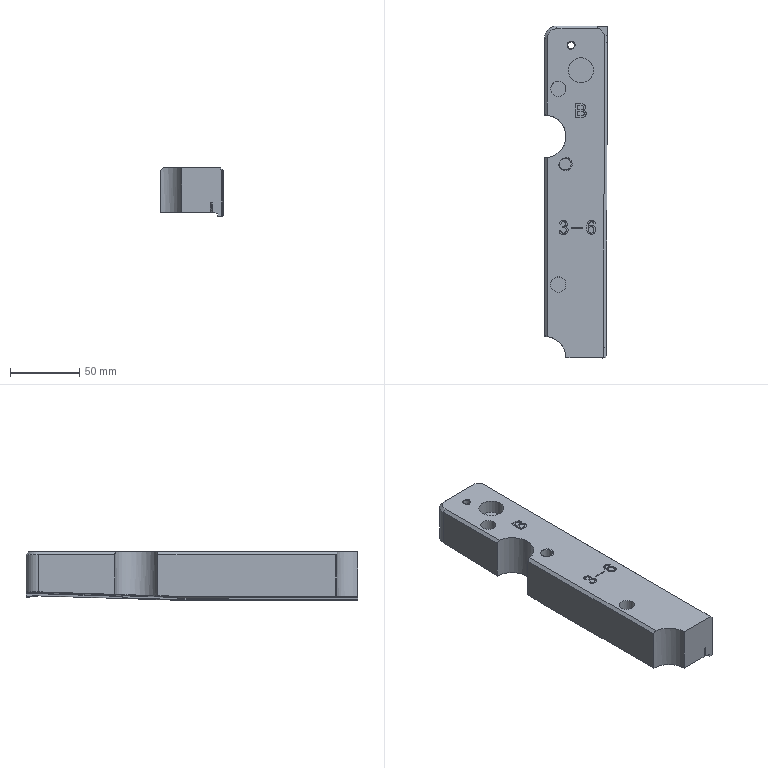NC program | NX | posted with a generic post | part box 45.476 x 239.737 x 35.001 mm
Lines 137 to 1068 of 14047:
(ZLEVEL_PROFILE , TOOL : D8R0.5)
N272 M6
N274 G53
N276 G17 G0 G90 X-123.905 Y28.641 S4500 M3
N278 G43 Z60. H0
N280 G94 G1 Z35.002 F4000.
N282 Z34.802 F1380.
N284 G3 X-120.891 Y25.655 R3.
N286 G1 X-119.898 Y25.659 F2300.
N288 X-119.885 Y25.662
N290 X-112.151 Y25.703
N292 X32.762 Y26.385
N294 X39.171 Y26.415 Z34.603 F100.
N296 X-112.151 Y25.703 F2300.
N298 X-119.885 Y25.662
N300 X-119.898 Y25.659
N302 X-120.891 Y25.655
N304 Z34.405 F100.
N306 X-119.89 Y25.662 F2300.
N308 X-112.153 Y25.703
N310 X-112.15
N312 X45.587 Y26.445
N314 X52.001 Y26.475 Z34.206 F100.
N316 X-112.15 Y25.703 F2300.
N318 X-112.153
N320 X-119.89 Y25.662
N322 X-120.891 Y25.655
N324 Z34.007 F100.
N326 X-119.89 Y25.662 F2300.
N328 X-112.153 Y25.703
N330 X-112.15
N332 X58.422 Y26.506
N334 X64.831 Y26.536 Z33.809 F100.
N336 X-112.15 Y25.703 F2300.
N338 X-112.153
N340 X-119.89 Y25.662
N342 X-120.891 Y25.655
N344 Z33.61 F100.
N346 X-119.89 Y25.662 F2300.
N348 X-112.153 Y25.703
N350 X-112.15
N352 X71.252 Y26.566
N354 X77.673 Y26.596 Z33.411 F100.
N356 X-112.15 Y25.703 F2300.
N358 X-112.153
N360 X-119.89 Y25.662
N362 X-120.891 Y25.655
N364 Z33.212 F100.
N366 X-119.89 Y25.662 F2300.
N368 X-112.153 Y25.703
N370 X-112.15
N372 X84.082 Y26.626
N374 G3 X87.068 Y29.64 R3.
N376 G1 Z33.412
N378 G0 Z60.
N380 X113.932 Y29.432
N382 G1 Z33.611 F4000.
N384 Z33.411 F1380.
N386 G3 X117.138 Y26.653 R3.
N388 G2 X119.632 Y26.738 R33.898 F2300.
N390 G1 X119.876
N392 G2 X123.869 Y22.744 R4.005
N394 G1 Y20.236
N396 G2 X123.582 Y18.314 R5.483
N398 X121.243 Y15.885 R4.013
N400 X116.883 Y17.033 R3.835
N402 X115.98 Y18.934 R4.396
N404 X114.06 Y19.41 R6.752
N406 X114.436 Y26.228 R3.615
N408 X116.388 Y26.591 R10.395
N410 X117.138 Y26.653 R33.898
N412 G1 X117.137 Y26.701 Z33.312 F100.
N414 X117.136 Y26.73 Z33.212
N416 G3 X114.789 Y26.601 R34.9 F2300.
N418 X112.765 Y26.236 R11.122
N420 X110.314 Y23.897 R3.595
N422 X112.79 Y19.251 R3.642
N424 G1 X113.253 Y19.112
N426 G3 X115.393 Y18.828 R13.686
N428 G2 X115.969 Y18.713 R2.024
N430 G3 X116.704 Y17.053 R4.135
N432 G1 X116.725 Y17.023
N434 G3 X123.156 Y17.227 R3.915
N436 X123.869 Y19.697 R4.438
N438 G1 Y22.744
N440 G3 X119.876 Y26.738 R4.005
N442 G1 X117.927
N444 G3 X117.136 Y26.73 R34.9
N446 G2 X114.073 Y29.666 R3.
N448 G1 Z33.412
N450 G0 Z33.611
N452 X-123.912 Y28.633
N454 G1 Z33.214 F4000.
N456 Z33.014 F1380.
N458 G3 X-120.891 Y25.655 R3.
N460 G1 X-119.89 Y25.662 F2300.
N462 X-112.153 Y25.703
N464 X-112.15
N466 X90.503 Y26.657
N468 G2 X103.915 Y26.501 R353.898
N470 X106.876 Y26.29 R36.623
N472 G1 X108.206 Y25.891
N474 G3 X109.592 Y25.363 R1.248
N476 G2 X111.274 Y26.29 R3.979
N478 X112.79 Y26.566 R9.709
N480 X116.229 Y26.738 R30.698
N482 G1 X119.876
N484 G2 X123.869 Y22.744 R4.005
N486 G1 Y19.437
N488 Y19.266 Z32.815 F100.
N490 Y22.744 F2300.
N492 G3 X119.876 Y26.738 R4.005
N494 G1 X114.527
N496 G3 X110.791 Y26.526 R28.567
N498 G1 X110.391 Y26.513
N500 X108.392 Y26.592
N502 G3 X96.912 Y26.687 R397.63
N504 G1 X-112.15 Y25.703
N506 X-112.153
N508 X-119.89 Y25.662
N510 X-120.891 Y25.655
N512 Z32.616 F100.
N514 X-119.89 Y25.662 F2300.
N516 X-112.153 Y25.703
N518 X-112.15
N520 X103.333 Y26.717
N522 G2 X110.791 Y26.683 R422.317
N524 X112.84 Y26.738 R49.109
N526 G1 X119.876
N528 G2 X123.869 Y22.744 R4.005
N530 G1 Y19.147
N532 Y19.053 Z32.418 F100.
N534 Y22.738 F2300.
N536 G3 X119.869 Y26.738 R4.
N538 G1 X107.859
N540 X-112.15 Y25.703
N542 X-112.153
N544 X-119.89 Y25.662
N546 X-120.891 Y25.655
N548 Z32.219 F100.
N550 X-119.89 Y25.662 F2300.
N552 X-112.153 Y25.703
N554 X-112.15
N556 X107.859 Y26.738
N558 X119.869
N560 G2 X123.869 Y22.738 R4.
N562 G1 Y19.011
N564 Y18.982 Z32.052 F100.
N566 Y22.738 F2300.
N568 G3 X119.869 Y26.738 R4.
N570 G1 X107.859
N572 X-112.15 Y25.703
N574 X-112.153
N576 X-119.89 Y25.662
N578 X-120.891 Y25.655
N580 Z31.886 F100.
N582 X-119.89 Y25.662 F2300.
N584 X-112.153 Y25.703
N586 X-112.15
N588 X107.859 Y26.738
N590 X119.869
N592 G2 X123.869 Y22.738 R4.
N594 G1 Y18.969
N596 Z31.719 F100.
N598 Y22.738 F2300.
N600 G3 X119.869 Y26.738 R4.
N602 G1 X107.859
N604 X-112.15 Y25.703
N606 X-112.153
N608 X-119.89 Y25.662
N610 X-120.891 Y25.655
N612 Z31.527 F100.
N614 X-119.89 Y25.662 F2300.
N616 X-112.153 Y25.703
N618 X-112.15
N620 X107.859 Y26.738
N622 X119.869
N624 G2 X123.869 Y22.738 R4.
N626 G1 Y18.969
N628 Z31.335 F100.
N630 Y22.738 F2300.
N632 G3 X119.869 Y26.738 R4.
N634 G1 X107.869
N636 X107.85
N638 X-112.15 Y25.703
N640 X-112.153
N642 X-119.89 Y25.662
N644 X-120.891 Y25.655
N646 Z31.143 F100.
N648 X-119.89 Y25.662 F2300.
N650 X-112.153 Y25.703
N652 X-112.15
N654 X107.85 Y26.738
N656 X107.869
N658 X119.869
N660 G2 X123.869 Y22.738 R4.
N662 G1 Y18.969
N664 Z30.951 F100.
N666 Y22.738 F2300.
N668 G3 X119.869 Y26.738 R4.
N670 G1 X107.869
N672 X107.85
N674 X-112.15 Y25.703
N676 X-112.153
N678 X-119.89 Y25.662
N680 X-120.891 Y25.655
N682 Z30.759 F100.
N684 X-119.89 Y25.662 F2300.
N686 X-112.153 Y25.703
N688 X-112.15
N690 X107.85 Y26.738
N692 X107.869
N694 X119.869
N696 G2 X123.869 Y22.738 R4.
N698 G1 Y18.969
N700 Z30.568 F100.
N702 Y22.738 F2300.
N704 G3 X119.869 Y26.738 R4.
N706 G1 X107.869
N708 X107.85
N710 X-112.15 Y25.703
N712 X-112.153
N714 X-119.89 Y25.662
N716 X-120.891 Y25.655
N718 Z30.376 F100.
N720 X-119.89 Y25.662 F2300.
N722 X-112.153 Y25.703
N724 X-112.15
N726 X107.85 Y26.738
N728 X107.869
N730 X119.869
N732 G2 X123.869 Y22.738 R4.
N734 G1 Y18.969
N736 X123.868 Y18.847 Z30.28 F100.
N738 X123.869 Y18.726 Z30.184
N740 Y22.738 F2300.
N742 G3 X119.869 Y26.738 R4.
N744 G1 X107.869
N746 X107.85
N748 X-112.15 Y25.703
N750 X-112.153
N752 X-119.89 Y25.662
N754 X-120.891 Y25.655
N756 Z29.992 F100.
N758 X-119.89 Y25.662 F2300.
N760 X-112.153 Y25.703
N762 X-112.15
N764 X107.85 Y26.738
N766 X107.869
N768 X119.869
N770 G2 X123.869 Y22.738 R4.
N772 G1 Y17.667
N774 Y16.591 Z29.8 F100.
N776 Y22.738 F2300.
N778 G3 X119.869 Y26.738 R4.
N780 G1 X107.869
N782 X107.85
N784 X-112.15 Y25.703
N786 X-112.153
N788 X-119.89 Y25.662
N790 X-120.891 Y25.655
N792 Z29.608 F100.
N794 X-119.89 Y25.662 F2300.
N796 X-112.153 Y25.703
N798 X-112.15
N800 X107.85 Y26.738
N802 X107.869
N804 X119.869
N806 G2 X123.869 Y22.738 R4.
N808 G1 Y15.342
N810 G2 X119.86 Y11.53 R4.009
N812 G1 X110.056
N814 X109.498 Z29.416 F100.
N816 X119.86 F2300.
N818 G3 X123.869 Y15.342 R4.009
N820 G1 Y22.738
N822 G3 X119.869 Y26.738 R4.
N824 G1 X107.869
N826 X107.85
N828 X-112.15 Y25.703
N830 X-112.153
N832 X-119.89 Y25.662
N834 X-120.891 Y25.655
N836 G2 X-123.912 Y28.634 R3.
N838 G1 Z29.616
N840 G0 Z60.
N842 X-111.361 Y-26.73
N844 G1 Z32.816 F4000.
N846 Z32.616 F1380.
N848 G3 X-108.366 Y-23.725 R3.
N850 G1 X-108.368 Y-22.722 F2300.
N852 G3 X-119.868 Y-11.238 R11.502
N854 G1 X-120.866 Y-11.236
N856 Z32.418 F100.
N858 X-119.868 Y-11.238 F2300.
N860 G2 X-108.368 Y-22.722 R11.502
N862 G1 X-108.366 Y-23.725
N864 Z32.219 F100.
N866 X-108.368 Y-22.722 F2300.
N868 G3 X-119.868 Y-11.238 R11.502
N870 G1 X-120.866 Y-11.236
N872 Z32.052 F100.
N874 X-119.868 Y-11.238 F2300.
N876 G2 X-108.368 Y-22.722 R11.502
N878 G1 X-108.366 Y-23.725
N880 Z31.886 F100.
N882 X-108.368 Y-22.722 F2300.
N884 G3 X-119.868 Y-11.238 R11.502
N886 G1 X-120.866 Y-11.236
N888 Z31.719 F100.
N890 X-119.868 Y-11.238 F2300.
N892 G2 X-108.368 Y-22.722 R11.502
N894 G1 X-108.366 Y-23.725
N896 Z31.527 F100.
N898 X-108.368 Y-22.759 F2300.
N900 X-108.369 Y-22.73
N902 G3 X-119.869 Y-11.238 R11.5
N904 G1 X-120.866 Y-11.236
N906 Z31.335 F100.
N908 X-119.869 Y-11.238 F2300.
N910 G2 X-108.369 Y-22.73 R11.5
N912 G1 X-108.368 Y-22.759
N914 X-108.366 Y-23.725
N916 Z31.143 F100.
N918 X-108.368 Y-22.759 F2300.
N920 X-108.369 Y-22.73
N922 G3 X-119.869 Y-11.238 R11.5
N924 G1 X-120.866 Y-11.236
N926 Z30.951 F100.
N928 X-119.869 Y-11.238 F2300.
N930 G2 X-108.369 Y-22.73 R11.5
N932 G1 X-108.368 Y-22.759
N934 X-108.366 Y-23.725
N936 Z30.759 F100.
N938 X-108.368 Y-22.759 F2300.
N940 X-108.369 Y-22.73
N942 G3 X-119.869 Y-11.238 R11.5
N944 G1 X-120.866 Y-11.236
N946 Z30.568 F100.
N948 X-119.869 Y-11.238 F2300.
N950 G2 X-108.369 Y-22.73 R11.5
N952 G1 X-108.368 Y-22.759
N954 X-108.366 Y-23.725
N956 Z30.376 F100.
N958 X-108.368 Y-22.759 F2300.
N960 X-108.369 Y-22.73
N962 G3 X-119.869 Y-11.238 R11.5
N964 G1 X-120.866 Y-11.236
N966 Z30.184 F100.
N968 X-119.869 Y-11.238 F2300.
N970 G2 X-108.369 Y-22.73 R11.5
N972 G1 X-108.368 Y-22.759
N974 X-108.366 Y-23.725
N976 Z29.992 F100.
N978 X-108.368 Y-22.759 F2300.
N980 X-108.369 Y-22.73
N982 G3 X-119.869 Y-11.238 R11.5
N984 G1 X-120.866 Y-11.236
N986 Z29.8 F100.
N988 X-119.869 Y-11.238 F2300.
N990 G2 X-108.369 Y-22.73 R11.5
N992 G1 X-108.368 Y-22.759
N994 X-108.366 Y-23.725
N996 Z29.608 F100.
N998 X-108.368 Y-22.759 F2300.
N1000 X-108.369 Y-22.73
N1002 G3 X-119.869 Y-11.238 R11.5
N1004 G1 X-120.866 Y-11.236
N1006 Z29.416 F100.
N1008 X-119.869 Y-11.238 F2300.
N1010 G2 X-108.369 Y-22.73 R11.5
N1012 G1 X-108.368 Y-22.759
N1014 X-108.366 Y-23.725
N1016 Z29.224 F100.
N1018 X-108.368 Y-22.759 F2300.
N1020 X-108.369 Y-22.73
N1022 G3 X-119.869 Y-11.238 R11.5
N1024 G1 X-120.866 Y-11.236
N1026 Z29.032 F100.
N1028 X-119.869 Y-11.238 F2300.
N1030 G2 X-108.369 Y-22.73 R11.5
N1032 G1 X-108.368 Y-22.759
N1034 X-108.366 Y-23.725
N1036 Z28.838 F100.
N1038 X-108.368 Y-22.759 F2300.
N1040 X-108.369 Y-22.73
N1042 G3 X-119.869 Y-11.238 R11.5
N1044 G1 X-120.866 Y-11.236
N1046 Z28.643 F100.
N1048 X-119.869 Y-11.238 F2300.
N1050 G2 X-108.369 Y-22.73 R11.5
N1052 G1 X-108.368 Y-22.759
N1054 X-108.366 Y-23.725
N1056 Z28.448 F100.
N1058 X-108.368 Y-22.759 F2300.
N1060 X-108.369 Y-22.73
N1062 G3 X-119.869 Y-11.238 R11.5
N1064 G1 X-120.866 Y-11.236
N1066 Z28.253 F100.
N1068 X-119.869 Y-11.238 F2300.
N1070 G2 X-108.369 Y-22.73 R11.5
N1072 G1 X-108.368 Y-22.759
N1074 X-108.366 Y-23.725
N1076 Z28.058 F100.
N1078 X-108.368 Y-22.759 F2300.
N1080 X-108.369 Y-22.73
N1082 G3 X-119.869 Y-11.238 R11.5
N1084 G1 X-120.866 Y-11.236
N1086 Z27.863 F100.
N1088 X-119.869 Y-11.238 F2300.
N1090 G2 X-108.369 Y-22.73 R11.5
N1092 G1 X-108.368 Y-22.759
N1094 X-108.366 Y-23.725
N1096 Z27.668 F100.
N1098 X-108.368 Y-22.759 F2300.
N1100 X-108.369 Y-22.73
N1102 G3 X-119.869 Y-11.238 R11.5
N1104 G1 X-120.866 Y-11.236
N1106 Z27.473 F100.
N1108 X-119.869 Y-11.238 F2300.
N1110 G2 X-108.369 Y-22.73 R11.5
N1112 G1 X-108.368 Y-22.759
N1114 X-108.366 Y-23.725
N1116 Z27.279 F100.
N1118 X-108.368 Y-22.759 F2300.
N1120 X-108.369 Y-22.73
N1122 G3 X-119.869 Y-11.238 R11.5
N1124 G1 X-120.866 Y-11.236
N1126 Z27.084 F100.
N1128 X-119.869 Y-11.238 F2300.
N1130 G2 X-108.369 Y-22.73 R11.5
N1132 G1 X-108.368 Y-22.759
N1134 X-108.366 Y-23.725
N1136 Z26.889 F100.
N1138 X-108.368 Y-22.759 F2300.
N1140 X-108.369 Y-22.73
N1142 G3 X-119.869 Y-11.238 R11.5
N1144 G1 X-120.866 Y-11.236
N1146 Z26.694 F100.
N1148 X-119.869 Y-11.238 F2300.
N1150 G2 X-108.369 Y-22.73 R11.5
N1152 G1 X-108.368 Y-22.759
N1154 X-108.366 Y-23.725
N1156 Z26.499 F100.
N1158 X-108.368 Y-22.759 F2300.
N1160 X-108.369 Y-22.73
N1162 G3 X-119.869 Y-11.238 R11.5
N1164 G1 X-120.866 Y-11.236
N1166 Z26.304 F100.
N1168 X-119.869 Y-11.238 F2300.
N1170 G2 X-108.369 Y-22.73 R11.5
N1172 G1 X-108.368 Y-22.759
N1174 X-108.366 Y-23.725
N1176 Z26.109 F100.
N1178 X-108.368 Y-22.759 F2300.
N1180 X-108.369 Y-22.73
N1182 G3 X-119.869 Y-11.238 R11.5
N1184 G1 X-120.866 Y-11.236
N1186 Z25.914 F100.
N1188 X-119.869 Y-11.238 F2300.
N1190 G2 X-108.369 Y-22.73 R11.5
N1192 G1 X-108.368 Y-22.759
N1194 X-108.366 Y-23.725
N1196 Z25.72 F100.
N1198 X-108.368 Y-22.759 F2300.
N1200 X-108.369 Y-22.73
N1202 G3 X-119.869 Y-11.238 R11.5
N1204 G1 X-120.866 Y-11.236
N1206 Z25.525 F100.
N1208 X-119.869 Y-11.238 F2300.
N1210 G2 X-108.369 Y-22.73 R11.5
N1212 G1 X-108.368 Y-22.759
N1214 X-108.366 Y-23.725
N1216 Z25.33 F100.
N1218 X-108.368 Y-22.759 F2300.
N1220 X-108.369 Y-22.73
N1222 G3 X-119.869 Y-11.238 R11.5
N1224 G1 X-120.866 Y-11.236
N1226 Z25.135 F100.
N1228 X-119.869 Y-11.238 F2300.
N1230 G2 X-108.369 Y-22.73 R11.5
N1232 G1 X-108.368 Y-22.759
N1234 X-108.366 Y-23.725
N1236 Z24.94 F100.
N1238 X-108.368 Y-22.759 F2300.
N1240 X-108.369 Y-22.73
N1242 G3 X-119.869 Y-11.238 R11.5
N1244 G1 X-120.866 Y-11.236
N1246 Z24.742 F100.
N1248 X-119.869 Y-11.238 F2300.
N1250 G2 X-108.369 Y-22.73 R11.5
N1252 G1 X-108.368 Y-22.759
N1254 X-108.366 Y-23.725
N1256 Z24.545 F100.
N1258 X-108.368 Y-22.759 F2300.
N1260 X-108.369 Y-22.73
N1262 G3 X-119.869 Y-11.238 R11.5
N1264 G1 X-120.866 Y-11.236
N1266 Z24.347 F100.
N1268 X-119.869 Y-11.238 F2300.
N1270 G2 X-108.369 Y-22.73 R11.5
N1272 G1 X-108.368 Y-22.759
N1274 X-108.366 Y-23.725
N1276 Z24.149 F100.
N1278 X-108.368 Y-22.759 F2300.
N1280 X-108.369 Y-22.73
N1282 G3 X-119.869 Y-11.238 R11.5
N1284 G1 X-120.866 Y-11.236
N1286 Z23.951 F100.
N1288 X-119.869 Y-11.238 F2300.
N1290 G2 X-108.369 Y-22.73 R11.5
N1292 G1 X-108.368 Y-22.759
N1294 X-108.366 Y-23.725
N1296 Z23.754 F100.
N1298 X-108.368 Y-22.759 F2300.
N1300 X-108.369 Y-22.73
N1302 G3 X-119.869 Y-11.238 R11.5
N1304 G1 X-120.866 Y-11.236
N1306 Z23.556 F100.
N1308 X-119.869 Y-11.238 F2300.
N1310 G2 X-108.369 Y-22.73 R11.5
N1312 G1 X-108.368 Y-22.759
N1314 X-108.366 Y-23.725
N1316 Z23.358 F100.
N1318 X-108.368 Y-22.759 F2300.
N1320 X-108.369 Y-22.73
N1322 G3 X-119.869 Y-11.238 R11.5
N1324 G1 X-120.866 Y-11.236
N1326 X-120.86 Z23.161 F100.
N1328 X-120.672 F2300.
N1330 X-119.869 Y-11.238
N1332 G2 X-108.369 Y-22.73 R11.5
N1334 G1 X-108.368 Y-22.759
N1336 X-108.366 Y-23.725
N1338 Z22.963 F100.
N1340 X-108.368 Y-22.759 F2300.
N1342 X-108.369 Y-22.73
N1344 G3 X-119.869 Y-11.238 R11.5
N1346 G1 X-120.672 Y-11.236
N1348 X-120.86
N1350 Z22.765 F100.
N1352 X-120.672 F2300.
N1354 X-119.869 Y-11.238
N1356 G2 X-108.369 Y-22.73 R11.5
N1358 G1 X-108.368 Y-22.759
N1360 X-108.366 Y-23.725
N1362 Z22.568 F100.
N1364 X-108.368 Y-22.759 F2300.
N1366 X-108.369 Y-22.73
N1368 G3 X-119.869 Y-11.238 R11.5
N1370 G1 X-120.86 Y-11.236
N1372 Z22.37 F100.
N1374 X-119.869 Y-11.238 F2300.
N1376 G2 X-108.369 Y-22.73 R11.5
N1378 G1 X-108.368 Y-22.759
N1380 X-108.366 Y-23.725
N1382 Z22.172 F100.
N1384 X-108.368 Y-22.759 F2300.
N1386 X-108.369 Y-22.73
N1388 G3 X-119.869 Y-11.238 R11.5
N1390 G1 X-120.86 Y-11.236
N1392 Z21.974 F100.
N1394 X-119.869 Y-11.238 F2300.
N1396 G2 X-108.369 Y-22.73 R11.5
N1398 G1 X-108.368 Y-22.759
N1400 X-108.366 Y-23.725
N1402 Z21.777 F100.
N1404 X-108.368 Y-22.759 F2300.
N1406 X-108.369 Y-22.73
N1408 G3 X-119.869 Y-11.238 R11.5
N1410 G1 X-120.86 Y-11.236
N1412 Z21.579 F100.
N1414 X-119.869 Y-11.238 F2300.
N1416 G2 X-108.369 Y-22.73 R11.5
N1418 G1 X-108.368 Y-22.759
N1420 X-108.366 Y-23.725
N1422 Z21.381 F100.
N1424 X-108.368 Y-22.759 F2300.
N1426 X-108.369 Y-22.73
N1428 G3 X-119.869 Y-11.238 R11.5
N1430 G1 X-120.86 Y-11.236
N1432 Z21.184 F100.
N1434 X-119.869 Y-11.238 F2300.
N1436 G2 X-108.369 Y-22.73 R11.5
N1438 G1 X-108.368 Y-22.759
N1440 X-108.366 Y-23.725
N1442 Z20.986 F100.
N1444 X-108.368 Y-22.759 F2300.
N1446 X-108.369 Y-22.73
N1448 G3 X-119.869 Y-11.238 R11.5
N1450 G1 X-120.86 Y-11.236
N1452 Z20.788 F100.
N1454 X-119.869 Y-11.238 F2300.
N1456 G2 X-108.369 Y-22.73 R11.5
N1458 G1 X-108.368 Y-22.759
N1460 X-108.366 Y-23.725
N1462 Z20.591 F100.
N1464 X-108.368 Y-22.759 F2300.
N1466 X-108.369 Y-22.73
N1468 G3 X-119.869 Y-11.238 R11.5
N1470 G1 X-120.86 Y-11.236
N1472 Z20.393 F100.
N1474 X-119.869 Y-11.238 F2300.
N1476 G2 X-108.369 Y-22.73 R11.5
N1478 G1 X-108.368 Y-22.759
N1480 X-108.366 Y-23.725
N1482 Z20.195 F100.
N1484 X-108.368 Y-22.759 F2300.
N1486 X-108.369 Y-22.73
N1488 G3 X-119.869 Y-11.238 R11.5
N1490 G1 X-120.86 Y-11.236
N1492 Z19.997 F100.
N1494 X-119.869 Y-11.238 F2300.
N1496 G2 X-108.369 Y-22.73 R11.5
N1498 G1 X-108.368 Y-22.759
N1500 X-108.366 Y-23.725
N1502 Z19.8 F100.
N1504 X-108.368 Y-22.759 F2300.
N1506 X-108.369 Y-22.73
N1508 G3 X-119.869 Y-11.238 R11.5
N1510 G1 X-120.86 Y-11.236
N1512 Z19.602 F100.
N1514 X-119.869 Y-11.238 F2300.
N1516 G2 X-108.369 Y-22.73 R11.5
N1518 G1 X-108.368 Y-22.759
N1520 X-108.366 Y-23.725
N1522 Z19.404 F100.
N1524 X-108.368 Y-22.759 F2300.
N1526 X-108.369 Y-22.73
N1528 G3 X-119.869 Y-11.238 R11.5
N1530 G1 X-120.86 Y-11.236
N1532 Z19.207 F100.
N1534 X-119.869 Y-11.238 F2300.
N1536 G2 X-108.369 Y-22.73 R11.5
N1538 G1 X-108.368 Y-22.759
N1540 X-108.366 Y-23.725
N1542 Z19.009 F100.
N1544 X-108.368 Y-22.759 F2300.
N1546 X-108.369 Y-22.73
N1548 G3 X-119.869 Y-11.238 R11.5
N1550 G1 X-120.86 Y-11.236
N1552 Z19. F100.
N1554 X-119.869 Y-11.238 F2300.
N1556 G2 X-108.369 Y-22.73 R11.5
N1558 G1 X-108.368 Y-22.759
N1560 X-108.366 Y-23.725
N1562 Z18.8 F100.
N1564 X-108.368 Y-22.759 F2300.
N1566 X-108.369 Y-22.73
N1568 G3 X-119.869 Y-11.238 R11.5
N1570 G1 X-120.86 Y-11.236
N1572 Z18.6 F100.
N1574 X-119.869 Y-11.238 F2300.
N1576 G2 X-108.369 Y-22.73 R11.5
N1578 G1 X-108.368 Y-22.759
N1580 X-108.366 Y-23.725
N1582 Z18.4 F100.
N1584 X-108.368 Y-22.759 F2300.
N1586 X-108.369 Y-22.73
N1588 G3 X-119.869 Y-11.238 R11.5
N1590 G1 X-120.86 Y-11.236
N1592 Z18.2 F100.
N1594 X-119.869 Y-11.238 F2300.
N1596 G2 X-108.369 Y-22.73 R11.5
N1598 G1 X-108.368 Y-22.759
N1600 X-108.366 Y-23.725
N1602 Z18. F100.
N1604 X-108.368 Y-22.759 F2300.
N1606 X-108.369 Y-22.73
N1608 G3 X-119.869 Y-11.238 R11.5
N1610 G1 X-120.86 Y-11.236
N1612 Z17.8 F100.
N1614 X-119.869 Y-11.238 F2300.
N1616 G2 X-108.369 Y-22.73 R11.5
N1618 G1 X-108.368 Y-22.759
N1620 X-108.366 Y-23.725
N1622 Z17.6 F100.
N1624 X-108.368 Y-22.759 F2300.
N1626 X-108.369 Y-22.73
N1628 G3 X-119.869 Y-11.238 R11.5
N1630 G1 X-120.86 Y-11.236
N1632 Z17.4 F100.
N1634 X-119.869 Y-11.238 F2300.
N1636 G2 X-108.369 Y-22.73 R11.5
N1638 G1 X-108.368 Y-22.759
N1640 X-108.366 Y-23.725
N1642 Z17.2 F100.
N1644 X-108.368 Y-22.759 F2300.
N1646 X-108.369 Y-22.73
N1648 G3 X-119.869 Y-11.238 R11.5
N1650 G1 X-120.86 Y-11.236
N1652 Z17. F100.
N1654 X-119.869 Y-11.238 F2300.
N1656 G2 X-108.369 Y-22.73 R11.5
N1658 G1 X-108.368 Y-22.759
N1660 X-108.366 Y-23.725
N1662 Z16.8 F100.
N1664 X-108.368 Y-22.759 F2300.
N1666 X-108.369 Y-22.73
N1668 G3 X-119.869 Y-11.238 R11.5
N1670 G1 X-120.86 Y-11.236
N1672 Z16.6 F100.
N1674 X-119.869 Y-11.238 F2300.
N1676 G2 X-108.369 Y-22.73 R11.5
N1678 G1 X-108.368 Y-22.759
N1680 X-108.366 Y-23.725
N1682 Z16.4 F100.
N1684 X-108.368 Y-22.759 F2300.
N1686 X-108.369 Y-22.73
N1688 G3 X-119.869 Y-11.238 R11.5
N1690 G1 X-120.86 Y-11.236
N1692 Z16.2 F100.
N1694 X-119.869 Y-11.238 F2300.
N1696 G2 X-108.369 Y-22.73 R11.5
N1698 G1 X-108.368 Y-22.759
N1700 X-108.366 Y-23.725
N1702 Z16. F100.
N1704 X-108.368 Y-22.759 F2300.
N1706 X-108.369 Y-22.73
N1708 G3 X-119.869 Y-11.238 R11.5
N1710 G1 X-120.86 Y-11.236
N1712 Z15.8 F100.
N1714 X-119.869 Y-11.238 F2300.
N1716 G2 X-108.369 Y-22.73 R11.5
N1718 G1 X-108.368 Y-22.759
N1720 X-108.366 Y-23.725
N1722 Z15.6 F100.
N1724 X-108.368 Y-22.759 F2300.
N1726 X-108.369 Y-22.73
N1728 G3 X-119.869 Y-11.238 R11.5
N1730 G1 X-120.86 Y-11.236
N1732 Z15.4 F100.
N1734 X-119.869 Y-11.238 F2300.
N1736 G2 X-108.369 Y-22.73 R11.5
N1738 G1 X-108.368 Y-22.759
N1740 X-108.366 Y-23.725
N1742 Z15.2 F100.
N1744 X-108.368 Y-22.759 F2300.
N1746 X-108.369 Y-22.73
N1748 G3 X-119.869 Y-11.238 R11.5
N1750 G1 X-120.86 Y-11.236
N1752 Z15. F100.
N1754 X-119.869 Y-11.238 F2300.
N1756 G2 X-108.369 Y-22.73 R11.5
N1758 G1 X-108.368 Y-22.759
N1760 X-108.366 Y-23.725
N1762 Z14.8 F100.
N1764 X-108.368 Y-22.759 F2300.
N1766 X-108.369 Y-22.73
N1768 G3 X-119.869 Y-11.238 R11.5
N1770 G1 X-120.86 Y-11.236
N1772 Z14.6 F100.
N1774 X-119.869 Y-11.238 F2300.
N1776 G2 X-108.369 Y-22.73 R11.5
N1778 G1 X-108.368 Y-22.759
N1780 X-108.366 Y-23.725
N1782 Z14.4 F100.
N1784 X-108.368 Y-22.759 F2300.
N1786 X-108.369 Y-22.73
N1788 G3 X-119.869 Y-11.238 R11.5
N1790 G1 X-120.86 Y-11.236
N1792 Z14.2 F100.
N1794 X-119.869 Y-11.238 F2300.
N1796 G2 X-108.369 Y-22.73 R11.5
N1798 G1 X-108.368 Y-22.759
N1800 X-108.366 Y-23.725
N1802 Z14. F100.
N1804 X-108.368 Y-22.759 F2300.
N1806 X-108.369 Y-22.73
N1808 G3 X-119.869 Y-11.238 R11.5
N1810 G1 X-120.86 Y-11.236
N1812 Z13.8 F100.
N1814 X-119.869 Y-11.238 F2300.
N1816 G2 X-108.369 Y-22.73 R11.5
N1818 G1 X-108.368 Y-22.759
N1820 X-108.366 Y-23.725
N1822 Z13.6 F100.
N1824 X-108.368 Y-22.759 F2300.
N1826 X-108.369 Y-22.73
N1828 G3 X-119.869 Y-11.238 R11.5
N1830 G1 X-120.86 Y-11.236
N1832 Z13.4 F100.
N1834 X-119.869 Y-11.238 F2300.
N1836 G2 X-108.369 Y-22.73 R11.5
N1838 G1 X-108.368 Y-22.759
N1840 X-108.366 Y-23.725
N1842 Z13.2 F100.
N1844 X-108.368 Y-22.759 F2300.
N1846 X-108.369 Y-22.73
N1848 G3 X-119.869 Y-11.238 R11.5
N1850 G1 X-120.86 Y-11.236
N1852 Z13. F100.
N1854 X-119.869 Y-11.238 F2300.
N1856 G2 X-108.369 Y-22.73 R11.5
N1858 G1 X-108.368 Y-22.759
N1860 X-108.366 Y-23.725
N1862 Z12.8 F100.
N1864 X-108.368 Y-22.759 F2300.
N1866 X-108.369 Y-22.73
N1868 G3 X-119.869 Y-11.238 R11.5
N1870 G1 X-120.86 Y-11.236
N1872 Z12.6 F100.
N1874 X-119.869 Y-11.238 F2300.
N1876 G2 X-108.369 Y-22.73 R11.5
N1878 G1 X-108.368 Y-22.759
N1880 X-108.366 Y-23.725
N1882 Z12.4 F100.
N1884 X-108.368 Y-22.759 F2300.
N1886 X-108.369 Y-22.73
N1888 G3 X-119.869 Y-11.238 R11.5
N1890 G1 X-120.86 Y-11.236
N1892 Z12.2 F100.
N1894 X-119.869 Y-11.238 F2300.
N1896 G2 X-108.369 Y-22.73 R11.5
N1898 G1 X-108.368 Y-22.759
N1900 X-108.366 Y-23.725
N1902 Z12. F100.
N1904 X-108.368 Y-22.759 F2300.
N1906 X-108.369 Y-22.73
N1908 G3 X-119.869 Y-11.238 R11.5
N1910 G1 X-120.86 Y-11.236
N1912 Z11.8 F100.
N1914 X-119.869 Y-11.238 F2300.
N1916 G2 X-108.369 Y-22.73 R11.5
N1918 G1 X-108.368 Y-22.759
N1920 X-108.366 Y-23.725
N1922 Z11.6 F100.
N1924 X-108.368 Y-22.759 F2300.
N1926 X-108.369 Y-22.73
N1928 G3 X-119.869 Y-11.238 R11.5
N1930 G1 X-120.86 Y-11.236
N1932 Z11.4 F100.
N1934 X-119.869 Y-11.238 F2300.
N1936 G2 X-108.369 Y-22.73 R11.5
N1938 G1 X-108.368 Y-22.759
N1940 X-108.366 Y-23.725
N1942 Z11.2 F100.
N1944 X-108.368 Y-22.759 F2300.
N1946 X-108.369 Y-22.73
N1948 G3 X-119.869 Y-11.238 R11.5
N1950 G1 X-120.86 Y-11.236
N1952 Z11. F100.
N1954 X-119.869 Y-11.238 F2300.
N1956 G2 X-108.369 Y-22.73 R11.5
N1958 G1 X-108.368 Y-22.759
N1960 X-108.366 Y-23.725
N1962 Z10.8 F100.
N1964 X-108.368 Y-22.759 F2300.
N1966 X-108.369 Y-22.73
N1968 G3 X-119.869 Y-11.238 R11.5
N1970 G1 X-120.86 Y-11.236
N1972 Z10.6 F100.
N1974 X-119.869 Y-11.238 F2300.
N1976 G2 X-108.369 Y-22.73 R11.5
N1978 G1 X-108.368 Y-22.759
N1980 X-108.366 Y-23.725
N1982 Z10.4 F100.
N1984 X-108.368 Y-22.759 F2300.
N1986 X-108.369 Y-22.73
N1988 G3 X-119.869 Y-11.238 R11.5
N1990 G1 X-120.86 Y-11.236
N1992 Z10.2 F100.
N1994 X-119.869 Y-11.238 F2300.
N1996 G2 X-108.369 Y-22.73 R11.5
N1998 G1 X-108.368 Y-22.759
N2000 X-108.366 Y-23.725
N2002 Z10. F100.
N2004 X-108.368 Y-22.759 F2300.
N2006 X-108.369 Y-22.73
N2008 G3 X-119.869 Y-11.238 R11.5
N2010 G1 X-120.86 Y-11.236
N2012 Z9.801 F100.
N2014 X-119.869 Y-11.238 F2300.
N2016 G2 X-108.369 Y-22.73 R11.5
N2018 G1 X-108.368 Y-22.759
N2020 X-108.366 Y-23.725
N2022 Z9.602 F100.
N2024 X-108.368 Y-22.759 F2300.
N2026 X-108.369 Y-22.73
N2028 G3 X-119.869 Y-11.238 R11.5
N2030 G1 X-120.86 Y-11.236
N2032 Z9.403 F100.
N2034 X-119.869 Y-11.238 F2300.
N2036 G2 X-108.369 Y-22.73 R11.5
N2038 G1 X-108.368 Y-22.759
N2040 X-108.366 Y-23.725
N2042 Z9.204 F100.
N2044 X-108.368 Y-22.759 F2300.
N2046 X-108.369 Y-22.73
N2048 G3 X-119.869 Y-11.238 R11.5
N2050 G1 X-120.86 Y-11.236
N2052 Z9.005 F100.
N2054 X-119.869 Y-11.238 F2300.
N2056 G2 X-108.369 Y-22.73 R11.5
N2058 G1 X-108.368 Y-22.759
N2060 X-108.366 Y-23.725
N2062 Z8.806 F100.
N2064 X-108.368 Y-22.759 F2300.
N2066 X-108.369 Y-22.73
N2068 G3 X-119.869 Y-11.238 R11.5
N2070 G1 X-120.86 Y-11.236
N2072 Z8.607 F100.
N2074 X-119.869 Y-11.238 F2300.
N2076 G2 X-108.369 Y-22.73 R11.5
N2078 G1 X-108.368 Y-22.759
N2080 X-108.366 Y-23.725
N2082 Z8.408 F100.
N2084 X-108.368 Y-22.759 F2300.
N2086 X-108.369 Y-22.73
N2088 G3 X-119.869 Y-11.238 R11.5
N2090 G1 X-120.86 Y-11.236
N2092 Z8.209 F100.
N2094 X-119.869 Y-11.238 F2300.
N2096 G2 X-108.369 Y-22.73 R11.5
N2098 G1 X-108.368 Y-22.759
N2100 X-108.366 Y-23.725
N2102 Z8.01 F100.
N2104 X-108.368 Y-22.759 F2300.
N2106 X-108.369 Y-22.73
N2108 G3 X-119.869 Y-11.238 R11.5
N2110 G1 X-120.86 Y-11.236
N2112 Z7.811 F100.
N2114 X-119.869 Y-11.238 F2300.
N2116 G2 X-108.369 Y-22.73 R11.5
N2118 G1 X-108.368 Y-22.759
N2120 X-108.366 Y-23.725
N2122 Z7.612 F100.
N2124 X-108.368 Y-22.759 F2300.
N2126 X-108.369 Y-22.73
N2128 G3 X-119.869 Y-11.238 R11.5